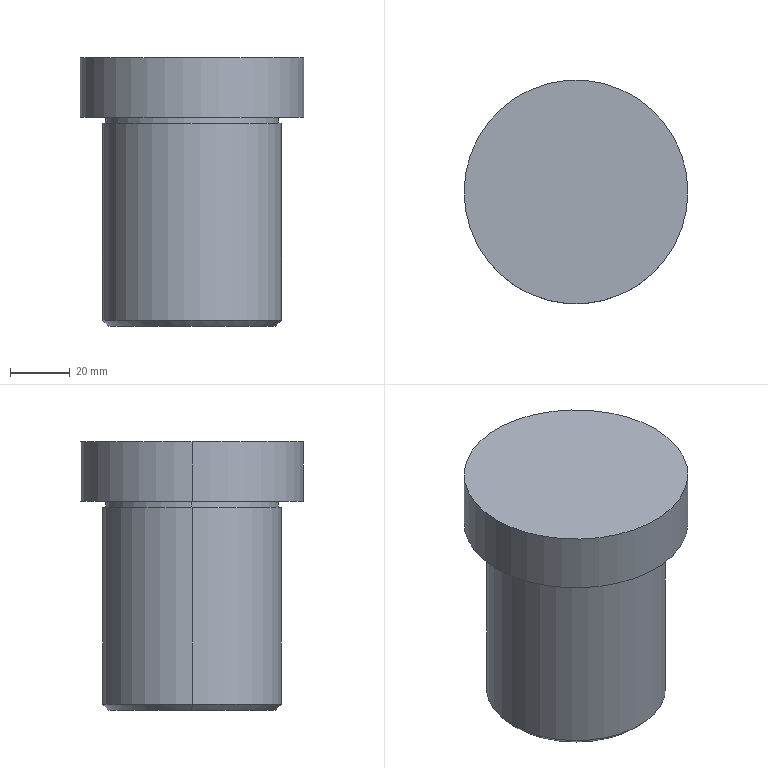Part | SolidWorks | features Chamfer 1, Extrusion 1, ICE 1, RefAxis 1, RevCut 1 | 1 solid | 12 faces | box 75 x 75 x 90 mm | volume 285538 mm3 | cylinder 6 | plane 4 | cone 2 | commonest cylinder face diameters 58 x2 60 x2 75 x2
STEP:
#1=CARTESIAN_POINT('',(37.5,0.,90.));
#2=VERTEX_POINT('',#1);
#3=CARTESIAN_POINT('',(-37.5,0.,90.));
#4=VERTEX_POINT('',#3);
#5=CARTESIAN_POINT('',(0.,0.,90.));
#6=DIRECTION('',(0.,0.,1.));
#7=DIRECTION('',(1.,0.,0.));
#8=AXIS2_PLACEMENT_3D('',#5,#6,#7);
#9=CIRCLE('',#8,37.5);
#10=EDGE_CURVE('',#2,#4,#9,.T.);
#11=ORIENTED_EDGE('',*,*,#10,.F.);
#12=CARTESIAN_POINT('',(37.5,0.,70.));
#13=VERTEX_POINT('',#12);
#14=CARTESIAN_POINT('',(37.5,0.,90.));
#15=DIRECTION('',(0.,0.,-1.));
#16=VECTOR('',#15,1000.);
#17=LINE('',#14,#16);
#18=EDGE_CURVE('',#2,#13,#17,.T.);
#19=ORIENTED_EDGE('',*,*,#18,.T.);
#20=CARTESIAN_POINT('',(-37.5,0.,70.));
#21=VERTEX_POINT('',#20);
#22=CARTESIAN_POINT('',(0.,0.,70.));
#23=DIRECTION('',(0.,0.,1.));
#24=DIRECTION('',(1.,0.,0.));
#25=AXIS2_PLACEMENT_3D('',#22,#23,#24);
#26=CIRCLE('',#25,37.5);
#27=EDGE_CURVE('',#13,#21,#26,.T.);
#28=ORIENTED_EDGE('',*,*,#27,.T.);
#29=CARTESIAN_POINT('',(-37.5,0.,90.));
#30=DIRECTION('',(0.,0.,-1.));
#31=VECTOR('',#30,1000.);
#32=LINE('',#29,#31);
#33=EDGE_CURVE('',#4,#21,#32,.T.);
#34=ORIENTED_EDGE('',*,*,#33,.F.);
#35=EDGE_LOOP('',(#11,#19,#28,#34));
#36=FACE_OUTER_BOUND('',#35,.T.);
#37=CARTESIAN_POINT('',(0.,0.,90.));
#38=DIRECTION('',(0.,0.,-1.));
#39=DIRECTION('',(-1.,0.,0.));
#40=AXIS2_PLACEMENT_3D('',#37,#38,#39);
#41=CYLINDRICAL_SURFACE('',#40,37.5);
#42=ADVANCED_FACE('',(#36),#41,.T.);
#43=CARTESIAN_POINT('',(29.,0.,68.));
#44=VERTEX_POINT('',#43);
#45=CARTESIAN_POINT('',(-29.,0.,68.));
#46=VERTEX_POINT('',#45);
#47=CARTESIAN_POINT('',(0.,0.,68.));
#48=DIRECTION('',(0.,0.,1.));
#49=DIRECTION('',(1.,0.,0.));
#50=AXIS2_PLACEMENT_3D('',#47,#48,#49);
#51=CIRCLE('',#50,29.);
#52=EDGE_CURVE('',#44,#46,#51,.T.);
#53=ORIENTED_EDGE('',*,*,#52,.T.);
#54=CARTESIAN_POINT('',(-29.,0.,70.));
#55=VERTEX_POINT('',#54);
#56=CARTESIAN_POINT('',(-29.,0.,70.));
#57=DIRECTION('',(0.,0.,1.));
#58=VECTOR('',#57,1000.);
#59=LINE('',#56,#58);
#60=EDGE_CURVE('',#46,#55,#59,.T.);
#61=ORIENTED_EDGE('',*,*,#60,.T.);
#62=CARTESIAN_POINT('',(29.,0.,70.));
#63=VERTEX_POINT('',#62);
#64=CARTESIAN_POINT('',(0.,0.,70.));
#65=DIRECTION('',(0.,0.,1.));
#66=DIRECTION('',(1.,0.,0.));
#67=AXIS2_PLACEMENT_3D('',#64,#65,#66);
#68=CIRCLE('',#67,29.);
#69=EDGE_CURVE('',#63,#55,#68,.T.);
#70=ORIENTED_EDGE('',*,*,#69,.F.);
#71=CARTESIAN_POINT('',(29.,0.,70.));
#72=DIRECTION('',(0.,0.,1.));
#73=VECTOR('',#72,1000.);
#74=LINE('',#71,#73);
#75=EDGE_CURVE('',#44,#63,#74,.T.);
#76=ORIENTED_EDGE('',*,*,#75,.F.);
#77=EDGE_LOOP('',(#53,#61,#70,#76));
#78=FACE_OUTER_BOUND('',#77,.T.);
#79=CARTESIAN_POINT('',(0.,0.,70.));
#80=DIRECTION('',(0.,0.,1.));
#81=DIRECTION('',(1.,0.,0.));
#82=AXIS2_PLACEMENT_3D('',#79,#80,#81);
#83=CYLINDRICAL_SURFACE('',#82,29.);
#84=ADVANCED_FACE('',(#78),#83,.T.);
#85=CARTESIAN_POINT('',(-28.,0.,0.));
#86=VERTEX_POINT('',#85);
#87=CARTESIAN_POINT('',(28.,0.,0.));
#88=VERTEX_POINT('',#87);
#89=CARTESIAN_POINT('',(0.,0.,0.));
#90=DIRECTION('',(0.,0.,-1.));
#91=DIRECTION('',(1.,0.,0.));
#92=AXIS2_PLACEMENT_3D('',#89,#90,#91);
#93=CIRCLE('',#92,28.);
#94=EDGE_CURVE('',#86,#88,#93,.T.);
#95=ORIENTED_EDGE('',*,*,#94,.F.);
#96=CARTESIAN_POINT('',(-30.,0.,2.));
#97=VERTEX_POINT('',#96);
#98=CARTESIAN_POINT('',(-30.,0.,2.));
#99=DIRECTION('',(-0.7071,0.,0.7071));
#100=VECTOR('',#99,1000.);
#101=LINE('',#98,#100);
#102=EDGE_CURVE('',#86,#97,#101,.T.);
#103=ORIENTED_EDGE('',*,*,#102,.T.);
#104=CARTESIAN_POINT('',(30.,0.,2.));
#105=VERTEX_POINT('',#104);
#106=CARTESIAN_POINT('',(0.,0.,2.));
#107=DIRECTION('',(0.,0.,1.));
#108=DIRECTION('',(1.,0.,0.));
#109=AXIS2_PLACEMENT_3D('',#106,#107,#108);
#110=CIRCLE('',#109,30.);
#111=EDGE_CURVE('',#105,#97,#110,.T.);
#112=ORIENTED_EDGE('',*,*,#111,.F.);
#113=CARTESIAN_POINT('',(30.,0.,2.));
#114=DIRECTION('',(0.7071,0.,0.7071));
#115=VECTOR('',#114,1000.);
#116=LINE('',#113,#115);
#117=EDGE_CURVE('',#88,#105,#116,.T.);
#118=ORIENTED_EDGE('',*,*,#117,.F.);
#119=EDGE_LOOP('',(#95,#103,#112,#118));
#120=FACE_OUTER_BOUND('',#119,.T.);
#121=CARTESIAN_POINT('',(0.,0.,2.));
#122=DIRECTION('',(0.,0.,1.));
#123=DIRECTION('',(1.,0.,0.));
#124=AXIS2_PLACEMENT_3D('',#121,#122,#123);
#125=CONICAL_SURFACE('',#124,30.,0.7854);
#126=ADVANCED_FACE('',(#120),#125,.T.);
#127=CARTESIAN_POINT('',(30.,0.,68.));
#128=VERTEX_POINT('',#127);
#129=CARTESIAN_POINT('',(-30.,0.,68.));
#130=VERTEX_POINT('',#129);
#131=CARTESIAN_POINT('',(0.,0.,68.));
#132=DIRECTION('',(0.,0.,1.));
#133=DIRECTION('',(1.,0.,0.));
#134=AXIS2_PLACEMENT_3D('',#131,#132,#133);
#135=CIRCLE('',#134,30.);
#136=EDGE_CURVE('',#128,#130,#135,.T.);
#137=ORIENTED_EDGE('',*,*,#136,.F.);
#138=CARTESIAN_POINT('',(30.,0.,70.));
#139=DIRECTION('',(0.,0.,-1.));
#140=VECTOR('',#139,1000.);
#141=LINE('',#138,#140);
#142=EDGE_CURVE('',#128,#105,#141,.T.);
#143=ORIENTED_EDGE('',*,*,#142,.T.);
#144=ORIENTED_EDGE('',*,*,#111,.T.);
#145=CARTESIAN_POINT('',(-30.,0.,70.));
#146=DIRECTION('',(0.,0.,-1.));
#147=VECTOR('',#146,1000.);
#148=LINE('',#145,#147);
#149=EDGE_CURVE('',#130,#97,#148,.T.);
#150=ORIENTED_EDGE('',*,*,#149,.F.);
#151=EDGE_LOOP('',(#137,#143,#144,#150));
#152=FACE_OUTER_BOUND('',#151,.T.);
#153=CARTESIAN_POINT('',(0.,0.,70.));
#154=DIRECTION('',(0.,0.,-1.));
#155=DIRECTION('',(-1.,0.,0.));
#156=AXIS2_PLACEMENT_3D('',#153,#154,#155);
#157=CYLINDRICAL_SURFACE('',#156,30.);
#158=ADVANCED_FACE('',(#152),#157,.T.);
#159=ORIENTED_EDGE('',*,*,#142,.F.);
#160=CARTESIAN_POINT('',(0.,0.,68.));
#161=DIRECTION('',(0.,0.,1.));
#162=DIRECTION('',(1.,0.,0.));
#163=AXIS2_PLACEMENT_3D('',#160,#161,#162);
#164=CIRCLE('',#163,30.);
#165=EDGE_CURVE('',#130,#128,#164,.T.);
#166=ORIENTED_EDGE('',*,*,#165,.F.);
#167=ORIENTED_EDGE('',*,*,#149,.T.);
#168=CARTESIAN_POINT('',(0.,0.,2.));
#169=DIRECTION('',(0.,0.,1.));
#170=DIRECTION('',(1.,0.,0.));
#171=AXIS2_PLACEMENT_3D('',#168,#169,#170);
#172=CIRCLE('',#171,30.);
#173=EDGE_CURVE('',#97,#105,#172,.T.);
#174=ORIENTED_EDGE('',*,*,#173,.T.);
#175=EDGE_LOOP('',(#159,#166,#167,#174));
#176=FACE_OUTER_BOUND('',#175,.T.);
#177=CARTESIAN_POINT('',(0.,0.,70.));
#178=DIRECTION('',(0.,0.,-1.));
#179=DIRECTION('',(-1.,0.,0.));
#180=AXIS2_PLACEMENT_3D('',#177,#178,#179);
#181=CYLINDRICAL_SURFACE('',#180,30.);
#182=ADVANCED_FACE('',(#176),#181,.T.);
#183=CARTESIAN_POINT('',(0.,0.,0.));
#184=DIRECTION('',(0.,0.,-1.));
#185=DIRECTION('',(1.,0.,0.));
#186=AXIS2_PLACEMENT_3D('',#183,#184,#185);
#187=CIRCLE('',#186,28.);
#188=EDGE_CURVE('',#88,#86,#187,.T.);
#189=ORIENTED_EDGE('',*,*,#188,.T.);
#190=ORIENTED_EDGE('',*,*,#94,.T.);
#191=EDGE_LOOP('',(#189,#190));
#192=FACE_OUTER_BOUND('',#191,.T.);
#193=CARTESIAN_POINT('',(0.,0.,0.));
#194=DIRECTION('',(0.,0.,1.));
#195=DIRECTION('',(1.,0.,0.));
#196=AXIS2_PLACEMENT_3D('',#193,#194,#195);
#197=PLANE('',#196);
#198=ADVANCED_FACE('',(#192),#197,.F.);
#199=ORIENTED_EDGE('',*,*,#102,.F.);
#200=ORIENTED_EDGE('',*,*,#188,.F.);
#201=ORIENTED_EDGE('',*,*,#117,.T.);
#202=ORIENTED_EDGE('',*,*,#173,.F.);
#203=EDGE_LOOP('',(#199,#200,#201,#202));
#204=FACE_OUTER_BOUND('',#203,.T.);
#205=CARTESIAN_POINT('',(0.,0.,2.));
#206=DIRECTION('',(0.,0.,1.));
#207=DIRECTION('',(1.,0.,0.));
#208=AXIS2_PLACEMENT_3D('',#205,#206,#207);
#209=CONICAL_SURFACE('',#208,30.,0.7854);
#210=ADVANCED_FACE('',(#204),#209,.T.);
#211=ORIENTED_EDGE('',*,*,#52,.F.);
#212=CARTESIAN_POINT('',(0.,0.,68.));
#213=DIRECTION('',(0.,0.,1.));
#214=DIRECTION('',(1.,0.,0.));
#215=AXIS2_PLACEMENT_3D('',#212,#213,#214);
#216=CIRCLE('',#215,29.);
#217=EDGE_CURVE('',#46,#44,#216,.T.);
#218=ORIENTED_EDGE('',*,*,#217,.F.);
#219=EDGE_LOOP('',(#211,#218));
#220=FACE_BOUND('',#219,.T.);
#221=ORIENTED_EDGE('',*,*,#165,.T.);
#222=ORIENTED_EDGE('',*,*,#136,.T.);
#223=EDGE_LOOP('',(#221,#222));
#224=FACE_OUTER_BOUND('',#223,.T.);
#225=CARTESIAN_POINT('',(30.,0.,68.));
#226=DIRECTION('',(0.,0.,-1.));
#227=DIRECTION('',(-1.,0.,0.));
#228=AXIS2_PLACEMENT_3D('',#225,#226,#227);
#229=PLANE('',#228);
#230=ADVANCED_FACE('',(#220,#224),#229,.F.);
#231=ORIENTED_EDGE('',*,*,#60,.F.);
#232=ORIENTED_EDGE('',*,*,#217,.T.);
#233=ORIENTED_EDGE('',*,*,#75,.T.);
#234=CARTESIAN_POINT('',(0.,0.,70.));
#235=DIRECTION('',(0.,0.,1.));
#236=DIRECTION('',(1.,0.,0.));
#237=AXIS2_PLACEMENT_3D('',#234,#235,#236);
#238=CIRCLE('',#237,29.);
#239=EDGE_CURVE('',#55,#63,#238,.T.);
#240=ORIENTED_EDGE('',*,*,#239,.F.);
#241=EDGE_LOOP('',(#231,#232,#233,#240));
#242=FACE_OUTER_BOUND('',#241,.T.);
#243=CARTESIAN_POINT('',(0.,0.,70.));
#244=DIRECTION('',(0.,0.,1.));
#245=DIRECTION('',(1.,0.,0.));
#246=AXIS2_PLACEMENT_3D('',#243,#244,#245);
#247=CYLINDRICAL_SURFACE('',#246,29.);
#248=ADVANCED_FACE('',(#242),#247,.T.);
#249=CARTESIAN_POINT('',(0.,0.,90.));
#250=DIRECTION('',(0.,0.,1.));
#251=DIRECTION('',(1.,0.,0.));
#252=AXIS2_PLACEMENT_3D('',#249,#250,#251);
#253=CIRCLE('',#252,37.5);
#254=EDGE_CURVE('',#4,#2,#253,.T.);
#255=ORIENTED_EDGE('',*,*,#254,.T.);
#256=ORIENTED_EDGE('',*,*,#10,.T.);
#257=EDGE_LOOP('',(#255,#256));
#258=FACE_OUTER_BOUND('',#257,.T.);
#259=CARTESIAN_POINT('',(0.,0.,90.));
#260=DIRECTION('',(0.,0.,1.));
#261=DIRECTION('',(1.,0.,0.));
#262=AXIS2_PLACEMENT_3D('',#259,#260,#261);
#263=PLANE('',#262);
#264=ADVANCED_FACE('',(#258),#263,.T.);
#265=ORIENTED_EDGE('',*,*,#18,.F.);
#266=ORIENTED_EDGE('',*,*,#254,.F.);
#267=ORIENTED_EDGE('',*,*,#33,.T.);
#268=CARTESIAN_POINT('',(0.,0.,70.));
#269=DIRECTION('',(0.,0.,1.));
#270=DIRECTION('',(1.,0.,0.));
#271=AXIS2_PLACEMENT_3D('',#268,#269,#270);
#272=CIRCLE('',#271,37.5);
#273=EDGE_CURVE('',#21,#13,#272,.T.);
#274=ORIENTED_EDGE('',*,*,#273,.T.);
#275=EDGE_LOOP('',(#265,#266,#267,#274));
#276=FACE_OUTER_BOUND('',#275,.T.);
#277=CARTESIAN_POINT('',(0.,0.,90.));
#278=DIRECTION('',(0.,0.,-1.));
#279=DIRECTION('',(-1.,0.,0.));
#280=AXIS2_PLACEMENT_3D('',#277,#278,#279);
#281=CYLINDRICAL_SURFACE('',#280,37.5);
#282=ADVANCED_FACE('',(#276),#281,.T.);
#283=ORIENTED_EDGE('',*,*,#273,.F.);
#284=ORIENTED_EDGE('',*,*,#27,.F.);
#285=EDGE_LOOP('',(#283,#284));
#286=FACE_OUTER_BOUND('',#285,.T.);
#287=ORIENTED_EDGE('',*,*,#69,.T.);
#288=ORIENTED_EDGE('',*,*,#239,.T.);
#289=EDGE_LOOP('',(#287,#288));
#290=FACE_BOUND('',#289,.T.);
#291=CARTESIAN_POINT('',(0.,0.,70.));
#292=DIRECTION('',(0.,0.,1.));
#293=DIRECTION('',(1.,0.,0.));
#294=AXIS2_PLACEMENT_3D('',#291,#292,#293);
#295=PLANE('',#294);
#296=ADVANCED_FACE('',(#286,#290),#295,.F.);
#297=CLOSED_SHELL('',(#42,#84,#126,#158,#182,#198,#210,#230,#248,#264,#282,#296));
#298=MANIFOLD_SOLID_BREP('',#297);
#299=CARTESIAN_POINT('',(0.,0.,0.));
#300=DIRECTION('',(0.,0.,1.));
#301=DIRECTION('',(1.,0.,0.));
#302=AXIS2_PLACEMENT_3D('',#299,#300,#301);
#303=(LENGTH_UNIT()NAMED_UNIT(*)SI_UNIT(.MILLI.,.METRE.));
#304=UNCERTAINTY_MEASURE_WITH_UNIT(LENGTH_MEASURE(0.00001),#303,'','');
#305=(NAMED_UNIT(*)PLANE_ANGLE_UNIT()SI_UNIT($,.RADIAN.));
#306=(NAMED_UNIT(*)SI_UNIT($,.STERADIAN.)SOLID_ANGLE_UNIT());
#307=(GEOMETRIC_REPRESENTATION_CONTEXT(3)GLOBAL_UNCERTAINTY_ASSIGNED_CONTEXT((#304))GLOBAL_UNIT_ASSIGNED_CONTEXT((#303,#305,#306))REPRESENTATION_CONTEXT('',''));
#308=ADVANCED_BREP_SHAPE_REPRESENTATION('',(#298,#302),#307);